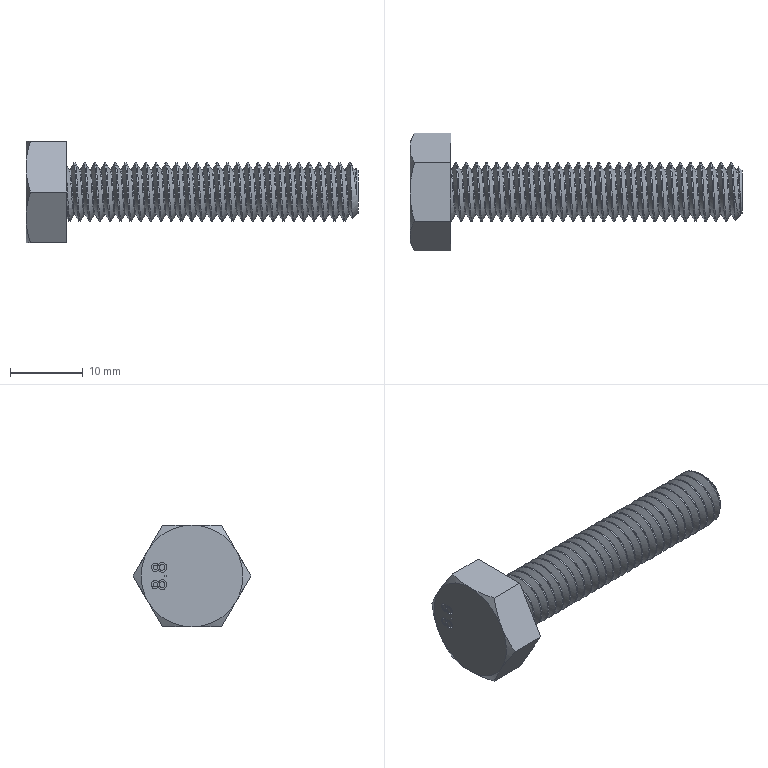Part | SolidWorks | features ICE 3, Chamfer 1, Extrusion 1, Helix 1, Revolution 1, Scale 1, SweepCut 1 | 1 solid | 120 faces | box 45.6 x 16.166 x 14 mm | volume 2539 mm3 | cylinder 57 | spline 35 | plane 20 | cone 8 | commonest cylinder face diameters 8 x57